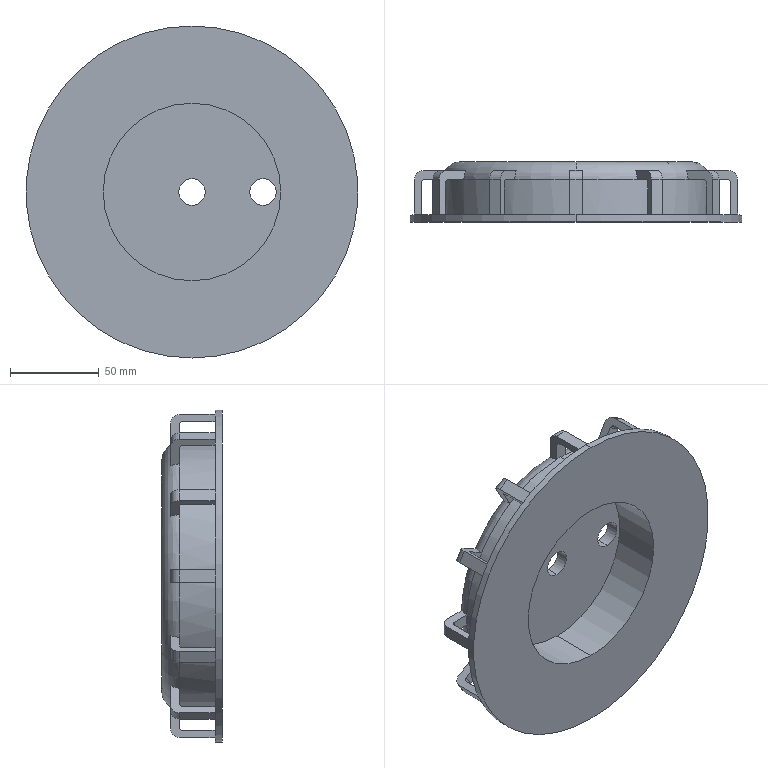Part | SolidWorks | features ICE 4, Fillet 3, CirPattern 1, Cut 1, Extrusion 1 | 1 solid | 112 faces | box 187 x 34 x 187 mm | volume 428914 mm3 | plane 76 | cylinder 34 | torus 2 | commonest cylinder face diameters 4 x12 10 x12 15 x4 100 x2 150 x2 187 x2